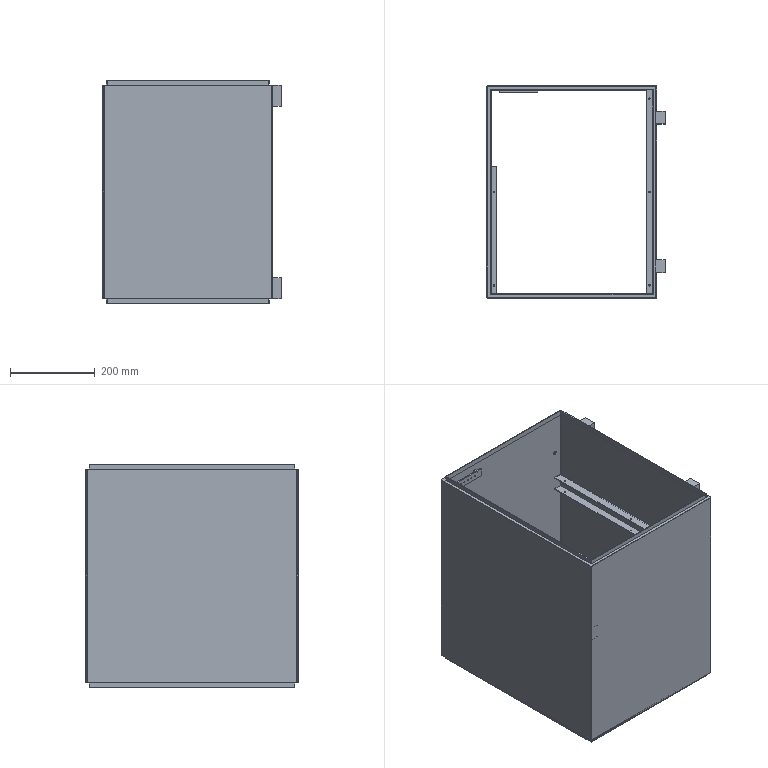Part | STEP file | Station three ctrl box body | 3 solids | 166 faces | box 420 x 500 x 524 mm | volume 2167031 mm3 | plane 90 | cylinder 76 | commonest cylinder face diameters 3.3 x48 5 x8 8.5 x8 10 x8 6 x4